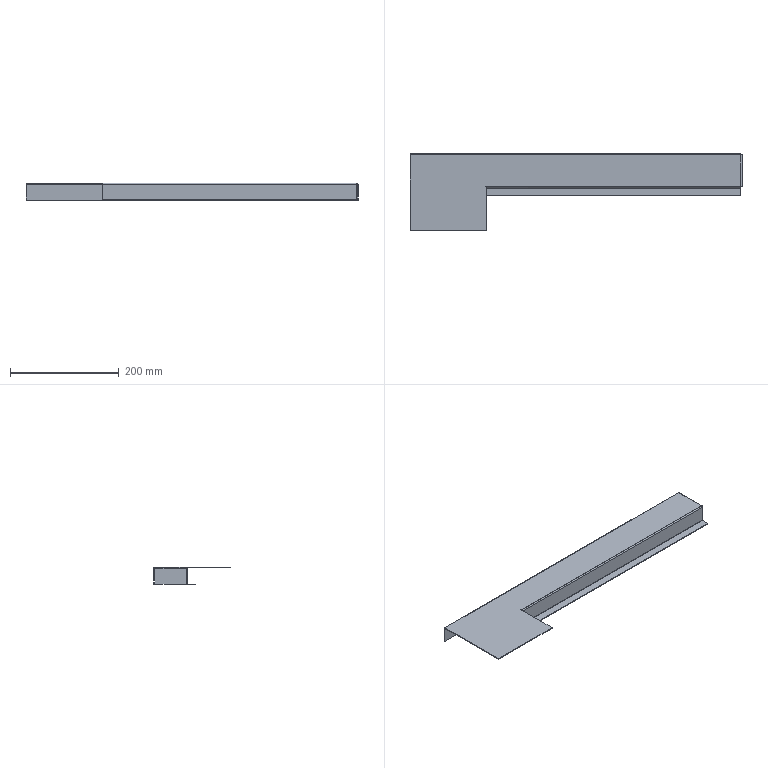Part | NX | 1 solid | 44 faces | box 611.5 x 141.5 x 33 mm | volume 135505 mm3 | plane 32 | cylinder 8 | spline 4 | commonest cylinder face diameters 1.473 x4 4.473 x4
STEP:
#1=CARTESIAN_POINT('',(304.293,-31.5,-30.763));
#2=VERTEX_POINT('',#1);
#3=CARTESIAN_POINT('',(304.293,-31.5,-2.237));
#4=VERTEX_POINT('',#3);
#5=CARTESIAN_POINT('',(304.293,-31.5,0.));
#6=DIRECTION('',(0.,0.,1.));
#7=VECTOR('',#6,1000.);
#8=LINE('',#5,#7);
#9=EDGE_CURVE('',#2,#4,#8,.T.);
#10=ORIENTED_EDGE('',*,*,#9,.F.);
#11=CARTESIAN_POINT('',(304.293,-30.,-30.763));
#12=VERTEX_POINT('',#11);
#13=CARTESIAN_POINT('',(304.293,-31.5,-30.763));
#14=DIRECTION('',(0.,1.,0.));
#15=VECTOR('',#14,1000.);
#16=LINE('',#13,#15);
#17=EDGE_CURVE('',#2,#12,#16,.T.);
#18=ORIENTED_EDGE('',*,*,#17,.T.);
#19=CARTESIAN_POINT('',(304.293,-30.,-2.237));
#20=VERTEX_POINT('',#19);
#21=CARTESIAN_POINT('',(304.293,-30.,-1.5));
#22=DIRECTION('',(0.,0.,-1.));
#23=VECTOR('',#22,1000.);
#24=LINE('',#21,#23);
#25=EDGE_CURVE('',#20,#12,#24,.T.);
#26=ORIENTED_EDGE('',*,*,#25,.F.);
#27=CARTESIAN_POINT('',(304.293,-30.,-2.237));
#28=DIRECTION('',(0.,1.,0.));
#29=VECTOR('',#28,1000.);
#30=LINE('',#27,#29);
#31=EDGE_CURVE('',#4,#20,#30,.T.);
#32=ORIENTED_EDGE('',*,*,#31,.F.);
#33=EDGE_LOOP('',(#10,#18,#26,#32));
#34=FACE_BOUND('',#33,.T.);
#35=CARTESIAN_POINT('',(304.293,-30.,-1.5));
#36=DIRECTION('',(1.,0.,0.));
#37=DIRECTION('',(0.,0.,-1.));
#38=AXIS2_PLACEMENT_3D('',#35,#36,#37);
#39=PLANE('',#38);
#40=ADVANCED_FACE('',(#34),#39,.T.);
#41=CARTESIAN_POINT('',(-165.,-31.5,-30.763));
#42=VERTEX_POINT('',#41);
#43=CARTESIAN_POINT('',(-165.,-31.5,-2.237));
#44=VERTEX_POINT('',#43);
#45=CARTESIAN_POINT('',(-165.,-31.5,-1.5));
#46=DIRECTION('',(0.,0.,1.));
#47=VECTOR('',#46,1000.);
#48=LINE('',#45,#47);
#49=EDGE_CURVE('',#42,#44,#48,.T.);
#50=ORIENTED_EDGE('',*,*,#49,.F.);
#51=CARTESIAN_POINT('',(304.293,-31.5,-30.763));
#52=DIRECTION('',(1.,0.,0.));
#53=VECTOR('',#52,1000.);
#54=LINE('',#51,#53);
#55=EDGE_CURVE('',#2,#42,#54,.F.);
#56=ORIENTED_EDGE('',*,*,#55,.F.);
#57=ORIENTED_EDGE('',*,*,#9,.T.);
#58=CARTESIAN_POINT('',(0.,-31.5,-2.237));
#59=DIRECTION('',(-1.,0.,0.));
#60=VECTOR('',#59,1000.);
#61=LINE('',#58,#60);
#62=EDGE_CURVE('',#4,#44,#61,.T.);
#63=ORIENTED_EDGE('',*,*,#62,.T.);
#64=EDGE_LOOP('',(#50,#56,#57,#63));
#65=FACE_BOUND('',#64,.T.);
#66=CARTESIAN_POINT('',(0.,-31.5,0.));
#67=DIRECTION('',(0.,-1.,0.));
#68=DIRECTION('',(0.,0.,-1.));
#69=AXIS2_PLACEMENT_3D('',#66,#67,#68);
#70=PLANE('',#69);
#71=ADVANCED_FACE('',(#65),#70,.T.);
#72=CARTESIAN_POINT('',(-165.,-30.,-30.763));
#73=VERTEX_POINT('',#72);
#74=CARTESIAN_POINT('',(304.293,-30.,-30.763));
#75=DIRECTION('',(1.,0.,0.));
#76=VECTOR('',#75,1000.);
#77=LINE('',#74,#76);
#78=EDGE_CURVE('',#12,#73,#77,.F.);
#79=ORIENTED_EDGE('',*,*,#78,.T.);
#80=CARTESIAN_POINT('',(-165.,-30.,-2.237));
#81=VERTEX_POINT('',#80);
#82=CARTESIAN_POINT('',(-165.,-30.,-1.5));
#83=DIRECTION('',(0.,0.,1.));
#84=VECTOR('',#83,1000.);
#85=LINE('',#82,#84);
#86=EDGE_CURVE('',#73,#81,#85,.T.);
#87=ORIENTED_EDGE('',*,*,#86,.T.);
#88=CARTESIAN_POINT('',(305.,-30.,-2.237));
#89=DIRECTION('',(-1.,0.,0.));
#90=VECTOR('',#89,1000.);
#91=LINE('',#88,#90);
#92=EDGE_CURVE('',#20,#81,#91,.T.);
#93=ORIENTED_EDGE('',*,*,#92,.F.);
#94=ORIENTED_EDGE('',*,*,#25,.T.);
#95=EDGE_LOOP('',(#79,#87,#93,#94));
#96=FACE_BOUND('',#95,.T.);
#97=CARTESIAN_POINT('',(0.,-30.,0.));
#98=DIRECTION('',(0.,-1.,0.));
#99=DIRECTION('',(0.,0.,-1.));
#100=AXIS2_PLACEMENT_3D('',#97,#98,#99);
#101=PLANE('',#100);
#102=ADVANCED_FACE('',(#96),#101,.F.);
#103=CARTESIAN_POINT('',(-305.,29.263,-1.5));
#104=VERTEX_POINT('',#103);
#105=CARTESIAN_POINT('',(-305.,-110.,-1.5));
#106=VERTEX_POINT('',#105);
#107=CARTESIAN_POINT('',(-305.,-30.,-1.5));
#108=DIRECTION('',(0.,-1.,0.));
#109=VECTOR('',#108,1000.);
#110=LINE('',#107,#109);
#111=EDGE_CURVE('',#104,#106,#110,.T.);
#112=ORIENTED_EDGE('',*,*,#111,.F.);
#113=CARTESIAN_POINT('',(304.263,29.263,-1.5));
#114=VERTEX_POINT('',#113);
#115=CARTESIAN_POINT('',(304.293,29.263,-1.5));
#116=DIRECTION('',(1.,0.,0.));
#117=VECTOR('',#116,1000.);
#118=LINE('',#115,#117);
#119=EDGE_CURVE('',#114,#104,#118,.F.);
#120=ORIENTED_EDGE('',*,*,#119,.F.);
#121=CARTESIAN_POINT('',(304.263,-29.263,-1.5));
#122=VERTEX_POINT('',#121);
#123=CARTESIAN_POINT('',(304.263,-29.293,-1.5));
#124=DIRECTION('',(0.,-1.,0.));
#125=VECTOR('',#124,1000.);
#126=LINE('',#123,#125);
#127=EDGE_CURVE('',#122,#114,#126,.F.);
#128=ORIENTED_EDGE('',*,*,#127,.F.);
#129=CARTESIAN_POINT('',(-165.,-29.263,-1.5));
#130=VERTEX_POINT('',#129);
#131=CARTESIAN_POINT('',(-165.,-29.263,-1.5));
#132=DIRECTION('',(-1.,0.,0.));
#133=VECTOR('',#132,1000.);
#134=LINE('',#131,#133);
#135=EDGE_CURVE('',#130,#122,#134,.F.);
#136=ORIENTED_EDGE('',*,*,#135,.F.);
#137=CARTESIAN_POINT('',(-165.,-28.513,-1.5));
#138=VERTEX_POINT('',#137);
#139=CARTESIAN_POINT('',(-165.,-28.513,-1.5));
#140=DIRECTION('',(0.,-1.,0.));
#141=VECTOR('',#140,1000.);
#142=LINE('',#139,#141);
#143=EDGE_CURVE('',#138,#130,#142,.T.);
#144=ORIENTED_EDGE('',*,*,#143,.F.);
#145=CARTESIAN_POINT('',(-165.75,-28.513,-1.5));
#146=VERTEX_POINT('',#145);
#147=CARTESIAN_POINT('',(-165.75,-28.513,-1.5));
#148=DIRECTION('',(1.,0.,0.));
#149=VECTOR('',#148,1000.);
#150=LINE('',#147,#149);
#151=EDGE_CURVE('',#146,#138,#150,.T.);
#152=ORIENTED_EDGE('',*,*,#151,.F.);
#153=CARTESIAN_POINT('',(-165.75,-30.,-1.5));
#154=VERTEX_POINT('',#153);
#155=CARTESIAN_POINT('',(-165.75,-30.,-1.5));
#156=DIRECTION('',(0.,1.,0.));
#157=VECTOR('',#156,1000.);
#158=LINE('',#155,#157);
#159=EDGE_CURVE('',#154,#146,#158,.T.);
#160=ORIENTED_EDGE('',*,*,#159,.F.);
#161=CARTESIAN_POINT('',(-165.,-30.,-1.5));
#162=VERTEX_POINT('',#161);
#163=CARTESIAN_POINT('',(-165.,-30.,-1.5));
#164=DIRECTION('',(-1.,0.,0.));
#165=VECTOR('',#164,1000.);
#166=LINE('',#163,#165);
#167=EDGE_CURVE('',#162,#154,#166,.T.);
#168=ORIENTED_EDGE('',*,*,#167,.F.);
#169=CARTESIAN_POINT('',(-165.,-110.,-1.5));
#170=VERTEX_POINT('',#169);
#171=CARTESIAN_POINT('',(-165.,-30.,-1.5));
#172=DIRECTION('',(0.,1.,0.));
#173=VECTOR('',#172,1000.);
#174=LINE('',#171,#173);
#175=EDGE_CURVE('',#170,#162,#174,.T.);
#176=ORIENTED_EDGE('',*,*,#175,.F.);
#177=CARTESIAN_POINT('',(-165.,-110.,-1.5));
#178=DIRECTION('',(1.,0.,0.));
#179=VECTOR('',#178,1000.);
#180=LINE('',#177,#179);
#181=EDGE_CURVE('',#106,#170,#180,.T.);
#182=ORIENTED_EDGE('',*,*,#181,.F.);
#183=EDGE_LOOP('',(#112,#120,#128,#136,#144,#152,#160,#168,#176,#182));
#184=FACE_BOUND('',#183,.T.);
#185=CARTESIAN_POINT('',(0.,0.,-1.5));
#186=DIRECTION('',(0.,0.,-1.));
#187=DIRECTION('',(-1.,0.,0.));
#188=AXIS2_PLACEMENT_3D('',#185,#186,#187);
#189=PLANE('',#188);
#190=ADVANCED_FACE('',(#184),#189,.T.);
#191=CARTESIAN_POINT('',(304.263,29.263,0.));
#192=VERTEX_POINT('',#191);
#193=CARTESIAN_POINT('',(-305.,29.263,0.));
#194=VERTEX_POINT('',#193);
#195=CARTESIAN_POINT('',(304.293,29.263,0.));
#196=DIRECTION('',(1.,0.,0.));
#197=VECTOR('',#196,1000.);
#198=LINE('',#195,#197);
#199=EDGE_CURVE('',#192,#194,#198,.F.);
#200=ORIENTED_EDGE('',*,*,#199,.T.);
#201=CARTESIAN_POINT('',(-305.,-110.,0.));
#202=VERTEX_POINT('',#201);
#203=CARTESIAN_POINT('',(-305.,-30.,0.));
#204=DIRECTION('',(0.,-1.,0.));
#205=VECTOR('',#204,1000.);
#206=LINE('',#203,#205);
#207=EDGE_CURVE('',#194,#202,#206,.T.);
#208=ORIENTED_EDGE('',*,*,#207,.T.);
#209=CARTESIAN_POINT('',(-165.,-110.,0.));
#210=VERTEX_POINT('',#209);
#211=CARTESIAN_POINT('',(-165.,-110.,0.));
#212=DIRECTION('',(1.,0.,0.));
#213=VECTOR('',#212,1000.);
#214=LINE('',#211,#213);
#215=EDGE_CURVE('',#202,#210,#214,.T.);
#216=ORIENTED_EDGE('',*,*,#215,.T.);
#217=CARTESIAN_POINT('',(-165.,-30.,0.));
#218=VERTEX_POINT('',#217);
#219=CARTESIAN_POINT('',(-165.,-30.,0.));
#220=DIRECTION('',(0.,1.,0.));
#221=VECTOR('',#220,1000.);
#222=LINE('',#219,#221);
#223=EDGE_CURVE('',#210,#218,#222,.T.);
#224=ORIENTED_EDGE('',*,*,#223,.T.);
#225=CARTESIAN_POINT('',(-165.75,-30.,0.));
#226=VERTEX_POINT('',#225);
#227=CARTESIAN_POINT('',(0.,-30.,0.));
#228=DIRECTION('',(1.,0.,0.));
#229=VECTOR('',#228,1000.);
#230=LINE('',#227,#229);
#231=EDGE_CURVE('',#226,#218,#230,.T.);
#232=ORIENTED_EDGE('',*,*,#231,.F.);
#233=CARTESIAN_POINT('',(-165.75,-28.513,0.));
#234=VERTEX_POINT('',#233);
#235=CARTESIAN_POINT('',(-165.75,0.,0.));
#236=DIRECTION('',(0.,-1.,0.));
#237=VECTOR('',#236,1000.);
#238=LINE('',#235,#237);
#239=EDGE_CURVE('',#234,#226,#238,.T.);
#240=ORIENTED_EDGE('',*,*,#239,.F.);
#241=CARTESIAN_POINT('',(-165.,-28.513,0.));
#242=VERTEX_POINT('',#241);
#243=CARTESIAN_POINT('',(0.,-28.513,0.));
#244=DIRECTION('',(-1.,0.,0.));
#245=VECTOR('',#244,1000.);
#246=LINE('',#243,#245);
#247=EDGE_CURVE('',#242,#234,#246,.T.);
#248=ORIENTED_EDGE('',*,*,#247,.F.);
#249=CARTESIAN_POINT('',(-165.,-29.263,0.));
#250=VERTEX_POINT('',#249);
#251=CARTESIAN_POINT('',(-165.,0.,0.));
#252=DIRECTION('',(0.,1.,0.));
#253=VECTOR('',#252,1000.);
#254=LINE('',#251,#253);
#255=EDGE_CURVE('',#250,#242,#254,.T.);
#256=ORIENTED_EDGE('',*,*,#255,.F.);
#257=CARTESIAN_POINT('',(304.263,-29.263,0.));
#258=VERTEX_POINT('',#257);
#259=CARTESIAN_POINT('',(-165.,-29.263,0.));
#260=DIRECTION('',(-1.,0.,0.));
#261=VECTOR('',#260,1000.);
#262=LINE('',#259,#261);
#263=EDGE_CURVE('',#250,#258,#262,.F.);
#264=ORIENTED_EDGE('',*,*,#263,.T.);
#265=CARTESIAN_POINT('',(304.263,-29.293,0.));
#266=DIRECTION('',(0.,-1.,0.));
#267=VECTOR('',#266,1000.);
#268=LINE('',#265,#267);
#269=EDGE_CURVE('',#258,#192,#268,.F.);
#270=ORIENTED_EDGE('',*,*,#269,.T.);
#271=EDGE_LOOP('',(#200,#208,#216,#224,#232,#240,#248,#256,#264,#270));
#272=FACE_BOUND('',#271,.T.);
#273=CARTESIAN_POINT('',(0.,0.,0.));
#274=DIRECTION('',(0.,0.,-1.));
#275=DIRECTION('',(-1.,0.,0.));
#276=AXIS2_PLACEMENT_3D('',#273,#274,#275);
#277=PLANE('',#276);
#278=ADVANCED_FACE('',(#272),#277,.F.);
#279=CARTESIAN_POINT('',(-305.,29.263,-1.5));
#280=DIRECTION('',(0.,0.,1.));
#281=VECTOR('',#280,1000.);
#282=LINE('',#279,#281);
#283=EDGE_CURVE('',#104,#194,#282,.T.);
#284=ORIENTED_EDGE('',*,*,#283,.F.);
#285=ORIENTED_EDGE('',*,*,#111,.T.);
#286=CARTESIAN_POINT('',(-305.,-110.,-1.5));
#287=DIRECTION('',(0.,0.,1.));
#288=VECTOR('',#287,1000.);
#289=LINE('',#286,#288);
#290=EDGE_CURVE('',#106,#202,#289,.T.);
#291=ORIENTED_EDGE('',*,*,#290,.T.);
#292=ORIENTED_EDGE('',*,*,#207,.F.);
#293=EDGE_LOOP('',(#284,#285,#291,#292));
#294=FACE_BOUND('',#293,.T.);
#295=CARTESIAN_POINT('',(-305.,-30.,-1.5));
#296=DIRECTION('',(-1.,0.,0.));
#297=DIRECTION('',(0.,0.,1.));
#298=AXIS2_PLACEMENT_3D('',#295,#296,#297);
#299=PLANE('',#298);
#300=ADVANCED_FACE('',(#294),#299,.T.);
#301=ORIENTED_EDGE('',*,*,#223,.F.);
#302=CARTESIAN_POINT('',(-165.,-110.,-1.5));
#303=DIRECTION('',(0.,0.,1.));
#304=VECTOR('',#303,1000.);
#305=LINE('',#302,#304);
#306=EDGE_CURVE('',#170,#210,#305,.T.);
#307=ORIENTED_EDGE('',*,*,#306,.F.);
#308=ORIENTED_EDGE('',*,*,#175,.T.);
#309=CARTESIAN_POINT('',(-165.,-30.,-1.5));
#310=DIRECTION('',(0.,0.,1.));
#311=VECTOR('',#310,1000.);
#312=LINE('',#309,#311);
#313=EDGE_CURVE('',#162,#218,#312,.T.);
#314=ORIENTED_EDGE('',*,*,#313,.T.);
#315=EDGE_LOOP('',(#301,#307,#308,#314));
#316=FACE_BOUND('',#315,.T.);
#317=CARTESIAN_POINT('',(-165.,-30.,-1.5));
#318=DIRECTION('',(1.,0.,0.));
#319=DIRECTION('',(0.,0.,-1.));
#320=AXIS2_PLACEMENT_3D('',#317,#318,#319);
#321=PLANE('',#320);
#322=ADVANCED_FACE('',(#316),#321,.T.);
#323=ORIENTED_EDGE('',*,*,#215,.F.);
#324=ORIENTED_EDGE('',*,*,#290,.F.);
#325=ORIENTED_EDGE('',*,*,#181,.T.);
#326=ORIENTED_EDGE('',*,*,#306,.T.);
#327=EDGE_LOOP('',(#323,#324,#325,#326));
#328=FACE_BOUND('',#327,.T.);
#329=CARTESIAN_POINT('',(-165.,-110.,-1.5));
#330=DIRECTION('',(0.,-1.,0.));
#331=DIRECTION('',(1.,0.,0.));
#332=AXIS2_PLACEMENT_3D('',#329,#330,#331);
#333=PLANE('',#332);
#334=ADVANCED_FACE('',(#328),#333,.T.);
#335=CARTESIAN_POINT('',(-165.75,-28.513,-1.5));
#336=DIRECTION('',(0.,0.,1.));
#337=VECTOR('',#336,1000.);
#338=LINE('',#335,#337);
#339=EDGE_CURVE('',#146,#234,#338,.T.);
#340=ORIENTED_EDGE('',*,*,#339,.T.);
#341=ORIENTED_EDGE('',*,*,#239,.T.);
#342=CARTESIAN_POINT('',(-165.75,-30.,-1.5));
#343=DIRECTION('',(0.,0.,1.));
#344=VECTOR('',#343,1000.);
#345=LINE('',#342,#344);
#346=EDGE_CURVE('',#154,#226,#345,.T.);
#347=ORIENTED_EDGE('',*,*,#346,.F.);
#348=ORIENTED_EDGE('',*,*,#159,.T.);
#349=EDGE_LOOP('',(#340,#341,#347,#348));
#350=FACE_BOUND('',#349,.T.);
#351=CARTESIAN_POINT('',(-165.75,-30.,-1.5));
#352=DIRECTION('',(1.,0.,0.));
#353=DIRECTION('',(0.,0.,-1.));
#354=AXIS2_PLACEMENT_3D('',#351,#352,#353);
#355=PLANE('',#354);
#356=ADVANCED_FACE('',(#350),#355,.T.);
#357=CARTESIAN_POINT('',(-165.,-28.513,-1.5));
#358=DIRECTION('',(0.,0.,1.));
#359=VECTOR('',#358,1000.);
#360=LINE('',#357,#359);
#361=EDGE_CURVE('',#138,#242,#360,.T.);
#362=ORIENTED_EDGE('',*,*,#361,.T.);
#363=ORIENTED_EDGE('',*,*,#247,.T.);
#364=ORIENTED_EDGE('',*,*,#339,.F.);
#365=ORIENTED_EDGE('',*,*,#151,.T.);
#366=EDGE_LOOP('',(#362,#363,#364,#365));
#367=FACE_BOUND('',#366,.T.);
#368=CARTESIAN_POINT('',(-165.75,-28.513,-1.5));
#369=DIRECTION('',(0.,-1.,0.));
#370=DIRECTION('',(0.,0.,-1.));
#371=AXIS2_PLACEMENT_3D('',#368,#369,#370);
#372=PLANE('',#371);
#373=ADVANCED_FACE('',(#367),#372,.T.);
#374=CARTESIAN_POINT('',(-165.,-29.263,-1.5));
#375=DIRECTION('',(0.,0.,1.));
#376=VECTOR('',#375,1000.);
#377=LINE('',#374,#376);
#378=EDGE_CURVE('',#130,#250,#377,.T.);
#379=ORIENTED_EDGE('',*,*,#378,.T.);
#380=ORIENTED_EDGE('',*,*,#255,.T.);
#381=ORIENTED_EDGE('',*,*,#361,.F.);
#382=ORIENTED_EDGE('',*,*,#143,.T.);
#383=EDGE_LOOP('',(#379,#380,#381,#382));
#384=FACE_BOUND('',#383,.T.);
#385=CARTESIAN_POINT('',(-165.,-28.513,-1.5));
#386=DIRECTION('',(-1.,0.,0.));
#387=DIRECTION('',(0.,0.,1.));
#388=AXIS2_PLACEMENT_3D('',#385,#386,#387);
#389=PLANE('',#388);
#390=ADVANCED_FACE('',(#384),#389,.T.);
#391=ORIENTED_EDGE('',*,*,#346,.T.);
#392=ORIENTED_EDGE('',*,*,#231,.T.);
#393=ORIENTED_EDGE('',*,*,#313,.F.);
#394=ORIENTED_EDGE('',*,*,#167,.T.);
#395=EDGE_LOOP('',(#391,#392,#393,#394));
#396=FACE_BOUND('',#395,.T.);
#397=CARTESIAN_POINT('',(-165.,-30.,-1.5));
#398=DIRECTION('',(0.,1.,0.));
#399=DIRECTION('',(0.,0.,1.));
#400=AXIS2_PLACEMENT_3D('',#397,#398,#399);
#401=PLANE('',#400);
#402=ADVANCED_FACE('',(#396),#401,.T.);
#403=ORIENTED_EDGE('',*,*,#31,.T.);
#404=CARTESIAN_POINT('',(304.263,-29.263,-1.5));
#405=CARTESIAN_POINT('',(304.273,-29.649,-1.5));
#406=CARTESIAN_POINT('',(304.283,-30.,-1.851));
#407=CARTESIAN_POINT('',(304.293,-30.,-2.237));
#408=B_SPLINE_CURVE_WITH_KNOTS('',3,(#404,#405,#406,#407),.UNSPECIFIED.,.F.,.F.,(4,4),(0.,1.),.UNSPECIFIED.);
#409=EDGE_CURVE('',#122,#20,#408,.T.);
#410=ORIENTED_EDGE('',*,*,#409,.F.);
#411=CARTESIAN_POINT('',(304.263,-29.263,-1.5));
#412=DIRECTION('',(0.,0.,1.));
#413=VECTOR('',#412,1000.);
#414=LINE('',#411,#413);
#415=EDGE_CURVE('',#122,#258,#414,.T.);
#416=ORIENTED_EDGE('',*,*,#415,.T.);
#417=CARTESIAN_POINT('',(304.263,-29.263,0.));
#418=CARTESIAN_POINT('',(304.268,-29.849,0.));
#419=CARTESIAN_POINT('',(304.278,-31.015,-0.4846));
#420=CARTESIAN_POINT('',(304.288,-31.5,-1.651));
#421=CARTESIAN_POINT('',(304.293,-31.5,-2.237));
#422=B_SPLINE_CURVE_WITH_KNOTS('',3,(#417,#418,#419,#420,#421),.UNSPECIFIED.,.F.,.F.,(4,1,4),(0.,0.5,1.),.UNSPECIFIED.);
#423=EDGE_CURVE('',#258,#4,#422,.T.);
#424=ORIENTED_EDGE('',*,*,#423,.T.);
#425=EDGE_LOOP('',(#403,#410,#416,#424));
#426=FACE_BOUND('',#425,.T.);
#427=CARTESIAN_POINT('',(304.263,-29.263,0.015));
#428=CARTESIAN_POINT('',(304.266,-29.558,0.015));
#429=CARTESIAN_POINT('',(304.268,-29.853,-0.0436));
#430=CARTESIAN_POINT('',(304.273,-30.397,-0.2692));
#431=CARTESIAN_POINT('',(304.276,-30.647,-0.4361));
#432=CARTESIAN_POINT('',(304.281,-31.064,-0.8529));
#433=CARTESIAN_POINT('',(304.283,-31.231,-1.103));
#434=CARTESIAN_POINT('',(304.288,-31.456,-1.647));
#435=CARTESIAN_POINT('',(304.29,-31.515,-1.942));
#436=CARTESIAN_POINT('',(304.293,-31.515,-2.237));
#437=CARTESIAN_POINT('',(304.263,-29.263,0.));
#438=CARTESIAN_POINT('',(304.266,-29.556,0.));
#439=CARTESIAN_POINT('',(304.268,-29.849,-0.05821));
#440=CARTESIAN_POINT('',(304.273,-30.39,-0.2823));
#441=CARTESIAN_POINT('',(304.276,-30.638,-0.4481));
#442=CARTESIAN_POINT('',(304.281,-31.052,-0.8621));
#443=CARTESIAN_POINT('',(304.283,-31.218,-1.11));
#444=CARTESIAN_POINT('',(304.288,-31.442,-1.651));
#445=CARTESIAN_POINT('',(304.29,-31.5,-1.944));
#446=CARTESIAN_POINT('',(304.293,-31.5,-2.237));
#447=CARTESIAN_POINT('',(304.263,-29.263,-1.5));
#448=CARTESIAN_POINT('',(304.266,-29.36,-1.5));
#449=CARTESIAN_POINT('',(304.268,-29.456,-1.519));
#450=CARTESIAN_POINT('',(304.273,-29.634,-1.593));
#451=CARTESIAN_POINT('',(304.276,-29.716,-1.648));
#452=CARTESIAN_POINT('',(304.281,-29.852,-1.784));
#453=CARTESIAN_POINT('',(304.283,-29.907,-1.866));
#454=CARTESIAN_POINT('',(304.288,-29.981,-2.044));
#455=CARTESIAN_POINT('',(304.29,-30.,-2.14));
#456=CARTESIAN_POINT('',(304.293,-30.,-2.237));
#457=CARTESIAN_POINT('',(304.263,-29.263,-1.515));
#458=CARTESIAN_POINT('',(304.266,-29.358,-1.515));
#459=CARTESIAN_POINT('',(304.268,-29.452,-1.534));
#460=CARTESIAN_POINT('',(304.273,-29.627,-1.606));
#461=CARTESIAN_POINT('',(304.276,-29.707,-1.66));
#462=CARTESIAN_POINT('',(304.281,-29.84,-1.793));
#463=CARTESIAN_POINT('',(304.283,-29.894,-1.873));
#464=CARTESIAN_POINT('',(304.288,-29.966,-2.048));
#465=CARTESIAN_POINT('',(304.29,-29.985,-2.142));
#466=CARTESIAN_POINT('',(304.293,-29.985,-2.237));
#467=B_SPLINE_SURFACE_WITH_KNOTS('',1,3,((#427,#428,#429,#430,#431,#432,#433,#434,#435,#436),(#437,#438,#439,#440,#441,#442,#443,#444,#445,#446),(#447,#448,#449,#450,#451,#452,#453,#454,#455,#456),(#457,#458,#459,#460,#461,#462,#463,#464,#465,#466)),.RULED_SURF.,.F.,.F.,.F.,(2,1,1,2),(4,2,2,2,4),(-0.01,0.,1.,1.01),(0.,0.25,0.5,0.75,1.),.UNSPECIFIED.);
#468=ADVANCED_FACE('',(#426),#467,.F.);
#469=CARTESIAN_POINT('',(-165.,-29.263,-2.237));
#470=DIRECTION('',(-1.,0.,0.));
#471=DIRECTION('',(0.,0.,1.));
#472=AXIS2_PLACEMENT_3D('',#469,#470,#471);
#473=CIRCLE('',#472,0.7366);
#474=EDGE_CURVE('',#81,#130,#473,.T.);
#475=ORIENTED_EDGE('',*,*,#474,.F.);
#476=CARTESIAN_POINT('',(-165.,-30.,-2.237));
#477=DIRECTION('',(0.,-1.,0.));
#478=VECTOR('',#477,1000.);
#479=LINE('',#476,#478);
#480=EDGE_CURVE('',#81,#44,#479,.T.);
#481=ORIENTED_EDGE('',*,*,#480,.T.);
#482=CARTESIAN_POINT('',(-165.,-29.263,-2.237));
#483=DIRECTION('',(-1.,0.,0.));
#484=DIRECTION('',(0.,0.,1.));
#485=AXIS2_PLACEMENT_3D('',#482,#483,#484);
#486=CIRCLE('',#485,2.237);
#487=EDGE_CURVE('',#44,#250,#486,.T.);
#488=ORIENTED_EDGE('',*,*,#487,.T.);
#489=ORIENTED_EDGE('',*,*,#378,.F.);
#490=EDGE_LOOP('',(#475,#481,#488,#489));
#491=FACE_BOUND('',#490,.T.);
#492=CARTESIAN_POINT('',(-165.,-29.263,-2.237));
#493=DIRECTION('',(1.,0.,0.));
#494=DIRECTION('',(0.,0.,-1.));
#495=AXIS2_PLACEMENT_3D('',#492,#493,#494);
#496=PLANE('',#495);
#497=ADVANCED_FACE('',(#491),#496,.F.);
#498=ORIENTED_EDGE('',*,*,#263,.F.);
#499=ORIENTED_EDGE('',*,*,#487,.F.);
#500=ORIENTED_EDGE('',*,*,#62,.F.);
#501=ORIENTED_EDGE('',*,*,#423,.F.);
#502=EDGE_LOOP('',(#498,#499,#500,#501));
#503=FACE_BOUND('',#502,.T.);
#504=CARTESIAN_POINT('',(-165.,-29.263,-2.237));
#505=DIRECTION('',(-1.,0.,0.));
#506=DIRECTION('',(0.,-1.,0.));
#507=AXIS2_PLACEMENT_3D('',#504,#505,#506);
#508=CYLINDRICAL_SURFACE('',#507,2.237);
#509=ADVANCED_FACE('',(#503),#508,.T.);
#510=ORIENTED_EDGE('',*,*,#135,.T.);
#511=ORIENTED_EDGE('',*,*,#409,.T.);
#512=ORIENTED_EDGE('',*,*,#92,.T.);
#513=ORIENTED_EDGE('',*,*,#474,.T.);
#514=EDGE_LOOP('',(#510,#511,#512,#513));
#515=FACE_BOUND('',#514,.T.);
#516=CARTESIAN_POINT('',(-165.,-29.263,-2.237));
#517=DIRECTION('',(-1.,0.,0.));
#518=DIRECTION('',(0.,-1.,0.));
#519=AXIS2_PLACEMENT_3D('',#516,#517,#518);
#520=CYLINDRICAL_SURFACE('',#519,0.7366);
#521=ADVANCED_FACE('',(#515),#520,.F.);
#522=CARTESIAN_POINT('',(-165.,-31.5,-30.763));
#523=DIRECTION('',(0.,1.,0.));
#524=VECTOR('',#523,1000.);
#525=LINE('',#522,#524);
#526=EDGE_CURVE('',#42,#73,#525,.T.);
#527=ORIENTED_EDGE('',*,*,#526,.F.);
#528=ORIENTED_EDGE('',*,*,#49,.T.);
#529=ORIENTED_EDGE('',*,*,#480,.F.);
#530=ORIENTED_EDGE('',*,*,#86,.F.);
#531=EDGE_LOOP('',(#527,#528,#529,#530));
#532=FACE_BOUND('',#531,.T.);
#533=CARTESIAN_POINT('',(-165.,-31.5,-1.5));
#534=DIRECTION('',(-1.,0.,0.));
#535=DIRECTION('',(0.,0.,1.));
#536=AXIS2_PLACEMENT_3D('',#533,#534,#535);
#537=PLANE('',#536);
#538=ADVANCED_FACE('',(#532),#537,.T.);
#539=CARTESIAN_POINT('',(306.5,29.293,-2.237));
#540=VERTEX_POINT('',#539);
#541=CARTESIAN_POINT('',(305.,29.293,-2.237));
#542=VERTEX_POINT('',#541);
#543=CARTESIAN_POINT('',(305.,29.293,-2.237));
#544=DIRECTION('',(-1.,0.,0.));
#545=VECTOR('',#544,1000.);
#546=LINE('',#543,#545);
#547=EDGE_CURVE('',#540,#542,#546,.T.);
#548=ORIENTED_EDGE('',*,*,#547,.T.);
#549=CARTESIAN_POINT('',(304.263,29.263,-1.5));
#550=CARTESIAN_POINT('',(304.649,29.273,-1.5));
#551=CARTESIAN_POINT('',(305.,29.283,-1.851));
#552=CARTESIAN_POINT('',(305.,29.293,-2.237));
#553=B_SPLINE_CURVE_WITH_KNOTS('',3,(#549,#550,#551,#552),.UNSPECIFIED.,.F.,.F.,(4,4),(0.,1.),.UNSPECIFIED.);
#554=EDGE_CURVE('',#114,#542,#553,.T.);
#555=ORIENTED_EDGE('',*,*,#554,.F.);
#556=CARTESIAN_POINT('',(304.263,29.263,-1.5));
#557=DIRECTION('',(0.,0.,1.));
#558=VECTOR('',#557,1000.);
#559=LINE('',#556,#558);
#560=EDGE_CURVE('',#114,#192,#559,.T.);
#561=ORIENTED_EDGE('',*,*,#560,.T.);
#562=CARTESIAN_POINT('',(304.263,29.263,0.));
#563=CARTESIAN_POINT('',(304.849,29.268,0.));
#564=CARTESIAN_POINT('',(306.015,29.278,-0.4846));
#565=CARTESIAN_POINT('',(306.5,29.288,-1.651));
#566=CARTESIAN_POINT('',(306.5,29.293,-2.237));
#567=B_SPLINE_CURVE_WITH_KNOTS('',3,(#562,#563,#564,#565,#566),.UNSPECIFIED.,.F.,.F.,(4,1,4),(0.,0.5,1.),.UNSPECIFIED.);
#568=EDGE_CURVE('',#192,#540,#567,.T.);
#569=ORIENTED_EDGE('',*,*,#568,.T.);
#570=EDGE_LOOP('',(#548,#555,#561,#569));
#571=FACE_BOUND('',#570,.T.);
#572=CARTESIAN_POINT('',(304.263,29.263,0.015));
#573=CARTESIAN_POINT('',(304.558,29.266,0.015));
#574=CARTESIAN_POINT('',(304.853,29.268,-0.0436));
#575=CARTESIAN_POINT('',(305.397,29.273,-0.2692));
#576=CARTESIAN_POINT('',(305.647,29.276,-0.4361));
#577=CARTESIAN_POINT('',(306.064,29.281,-0.8529));
#578=CARTESIAN_POINT('',(306.231,29.283,-1.103));
#579=CARTESIAN_POINT('',(306.456,29.288,-1.647));
#580=CARTESIAN_POINT('',(306.515,29.29,-1.942));
#581=CARTESIAN_POINT('',(306.515,29.293,-2.237));
#582=CARTESIAN_POINT('',(304.263,29.263,0.));
#583=CARTESIAN_POINT('',(304.556,29.266,0.));
#584=CARTESIAN_POINT('',(304.849,29.268,-0.05821));
#585=CARTESIAN_POINT('',(305.39,29.273,-0.2823));
#586=CARTESIAN_POINT('',(305.638,29.276,-0.4481));
#587=CARTESIAN_POINT('',(306.052,29.281,-0.8621));
#588=CARTESIAN_POINT('',(306.218,29.283,-1.11));
#589=CARTESIAN_POINT('',(306.442,29.288,-1.651));
#590=CARTESIAN_POINT('',(306.5,29.29,-1.944));
#591=CARTESIAN_POINT('',(306.5,29.293,-2.237));
#592=CARTESIAN_POINT('',(304.263,29.263,-1.5));
#593=CARTESIAN_POINT('',(304.36,29.266,-1.5));
#594=CARTESIAN_POINT('',(304.456,29.268,-1.519));
#595=CARTESIAN_POINT('',(304.634,29.273,-1.593));
#596=CARTESIAN_POINT('',(304.716,29.276,-1.648));
#597=CARTESIAN_POINT('',(304.852,29.281,-1.784));
#598=CARTESIAN_POINT('',(304.907,29.283,-1.866));
#599=CARTESIAN_POINT('',(304.981,29.288,-2.044));
#600=CARTESIAN_POINT('',(305.,29.29,-2.14));
#601=CARTESIAN_POINT('',(305.,29.293,-2.237));
#602=CARTESIAN_POINT('',(304.263,29.263,-1.515));
#603=CARTESIAN_POINT('',(304.358,29.266,-1.515));
#604=CARTESIAN_POINT('',(304.452,29.268,-1.534));
#605=CARTESIAN_POINT('',(304.627,29.273,-1.606));
#606=CARTESIAN_POINT('',(304.707,29.276,-1.66));
#607=CARTESIAN_POINT('',(304.84,29.281,-1.793));
#608=CARTESIAN_POINT('',(304.894,29.283,-1.873));
#609=CARTESIAN_POINT('',(304.966,29.288,-2.048));
#610=CARTESIAN_POINT('',(304.985,29.29,-2.142));
#611=CARTESIAN_POINT('',(304.985,29.293,-2.237));
#612=B_SPLINE_SURFACE_WITH_KNOTS('',1,3,((#572,#573,#574,#575,#576,#577,#578,#579,#580,#581),(#582,#583,#584,#585,#586,#587,#588,#589,#590,#591),(#592,#593,#594,#595,#596,#597,#598,#599,#600,#601),(#602,#603,#604,#605,#606,#607,#608,#609,#610,#611)),.RULED_SURF.,.F.,.F.,.F.,(2,1,1,2),(4,2,2,2,4),(-0.01,0.,1.,1.01),(0.,0.25,0.5,0.75,1.),.UNSPECIFIED.);
#613=ADVANCED_FACE('',(#571),#612,.F.);
#614=CARTESIAN_POINT('',(305.,-29.293,-2.237));
#615=VERTEX_POINT('',#614);
#616=CARTESIAN_POINT('',(305.,-29.293,-2.237));
#617=CARTESIAN_POINT('',(305.,-29.283,-1.851));
#618=CARTESIAN_POINT('',(304.649,-29.273,-1.5));
#619=CARTESIAN_POINT('',(304.263,-29.263,-1.5));
#620=B_SPLINE_CURVE_WITH_KNOTS('',3,(#616,#617,#618,#619),.UNSPECIFIED.,.F.,.F.,(4,4),(0.,1.),.UNSPECIFIED.);
#621=EDGE_CURVE('',#615,#122,#620,.T.);
#622=ORIENTED_EDGE('',*,*,#621,.F.);
#623=CARTESIAN_POINT('',(306.5,-29.293,-2.237));
#624=VERTEX_POINT('',#623);
#625=CARTESIAN_POINT('',(305.,-29.293,-2.237));
#626=DIRECTION('',(-1.,0.,0.));
#627=VECTOR('',#626,1000.);
#628=LINE('',#625,#627);
#629=EDGE_CURVE('',#624,#615,#628,.T.);
#630=ORIENTED_EDGE('',*,*,#629,.F.);
#631=CARTESIAN_POINT('',(306.5,-29.293,-2.237));
#632=CARTESIAN_POINT('',(306.5,-29.288,-1.651));
#633=CARTESIAN_POINT('',(306.015,-29.278,-0.4846));
#634=CARTESIAN_POINT('',(304.849,-29.268,0.));
#635=CARTESIAN_POINT('',(304.263,-29.263,0.));
#636=B_SPLINE_CURVE_WITH_KNOTS('',3,(#631,#632,#633,#634,#635),.UNSPECIFIED.,.F.,.F.,(4,1,4),(0.,0.5,1.),.UNSPECIFIED.);
#637=EDGE_CURVE('',#624,#258,#636,.T.);
#638=ORIENTED_EDGE('',*,*,#637,.T.);
#639=ORIENTED_EDGE('',*,*,#415,.F.);
#640=EDGE_LOOP('',(#622,#630,#638,#639));
#641=FACE_BOUND('',#640,.T.);
#642=CARTESIAN_POINT('',(306.515,-29.293,-2.237));
#643=CARTESIAN_POINT('',(306.515,-29.29,-1.942));
#644=CARTESIAN_POINT('',(306.456,-29.288,-1.647));
#645=CARTESIAN_POINT('',(306.231,-29.283,-1.103));
#646=CARTESIAN_POINT('',(306.064,-29.281,-0.8529));
#647=CARTESIAN_POINT('',(305.647,-29.276,-0.4361));
#648=CARTESIAN_POINT('',(305.397,-29.273,-0.2692));
#649=CARTESIAN_POINT('',(304.853,-29.268,-0.0436));
#650=CARTESIAN_POINT('',(304.558,-29.266,0.015));
#651=CARTESIAN_POINT('',(304.263,-29.263,0.015));
#652=CARTESIAN_POINT('',(306.5,-29.293,-2.237));
#653=CARTESIAN_POINT('',(306.5,-29.29,-1.944));
#654=CARTESIAN_POINT('',(306.442,-29.288,-1.651));
#655=CARTESIAN_POINT('',(306.218,-29.283,-1.11));
#656=CARTESIAN_POINT('',(306.052,-29.281,-0.8621));
#657=CARTESIAN_POINT('',(305.638,-29.276,-0.4481));
#658=CARTESIAN_POINT('',(305.39,-29.273,-0.2823));
#659=CARTESIAN_POINT('',(304.849,-29.268,-0.05821));
#660=CARTESIAN_POINT('',(304.556,-29.266,0.));
#661=CARTESIAN_POINT('',(304.263,-29.263,0.));
#662=CARTESIAN_POINT('',(305.,-29.293,-2.237));
#663=CARTESIAN_POINT('',(305.,-29.29,-2.14));
#664=CARTESIAN_POINT('',(304.981,-29.288,-2.044));
#665=CARTESIAN_POINT('',(304.907,-29.283,-1.866));
#666=CARTESIAN_POINT('',(304.852,-29.281,-1.784));
#667=CARTESIAN_POINT('',(304.716,-29.276,-1.648));
#668=CARTESIAN_POINT('',(304.634,-29.273,-1.593));
#669=CARTESIAN_POINT('',(304.456,-29.268,-1.519));
#670=CARTESIAN_POINT('',(304.36,-29.266,-1.5));
#671=CARTESIAN_POINT('',(304.263,-29.263,-1.5));
#672=CARTESIAN_POINT('',(304.985,-29.293,-2.237));
#673=CARTESIAN_POINT('',(304.985,-29.29,-2.142));
#674=CARTESIAN_POINT('',(304.966,-29.288,-2.048));
#675=CARTESIAN_POINT('',(304.894,-29.283,-1.873));
#676=CARTESIAN_POINT('',(304.84,-29.281,-1.793));
#677=CARTESIAN_POINT('',(304.707,-29.276,-1.66));
#678=CARTESIAN_POINT('',(304.627,-29.273,-1.606));
#679=CARTESIAN_POINT('',(304.452,-29.268,-1.534));
#680=CARTESIAN_POINT('',(304.358,-29.266,-1.515));
#681=CARTESIAN_POINT('',(304.263,-29.263,-1.515));
#682=B_SPLINE_SURFACE_WITH_KNOTS('',1,3,((#642,#643,#644,#645,#646,#647,#648,#649,#650,#651),(#652,#653,#654,#655,#656,#657,#658,#659,#660,#661),(#662,#663,#664,#665,#666,#667,#668,#669,#670,#671),(#672,#673,#674,#675,#676,#677,#678,#679,#680,#681)),.RULED_SURF.,.F.,.F.,.F.,(2,1,1,2),(4,2,2,2,4),(-0.01,0.,1.,1.01),(0.,0.25,0.5,0.75,1.),.UNSPECIFIED.);
#683=ADVANCED_FACE('',(#641),#682,.F.);
#684=ORIENTED_EDGE('',*,*,#269,.F.);
#685=ORIENTED_EDGE('',*,*,#637,.F.);
#686=CARTESIAN_POINT('',(306.5,0.,-2.237));
#687=DIRECTION('',(0.,1.,0.));
#688=VECTOR('',#687,1000.);
#689=LINE('',#686,#688);
#690=EDGE_CURVE('',#624,#540,#689,.T.);
#691=ORIENTED_EDGE('',*,*,#690,.T.);
#692=ORIENTED_EDGE('',*,*,#568,.F.);
#693=EDGE_LOOP('',(#684,#685,#691,#692));
#694=FACE_BOUND('',#693,.T.);
#695=CARTESIAN_POINT('',(304.263,-29.293,-2.237));
#696=DIRECTION('',(0.,-1.,0.));
#697=DIRECTION('',(1.,0.,0.));
#698=AXIS2_PLACEMENT_3D('',#695,#696,#697);
#699=CYLINDRICAL_SURFACE('',#698,2.237);
#700=ADVANCED_FACE('',(#694),#699,.T.);
#701=ORIENTED_EDGE('',*,*,#127,.T.);
#702=ORIENTED_EDGE('',*,*,#554,.T.);
#703=CARTESIAN_POINT('',(305.,30.,-2.237));
#704=DIRECTION('',(0.,-1.,0.));
#705=VECTOR('',#704,1000.);
#706=LINE('',#703,#705);
#707=EDGE_CURVE('',#542,#615,#706,.T.);
#708=ORIENTED_EDGE('',*,*,#707,.T.);
#709=ORIENTED_EDGE('',*,*,#621,.T.);
#710=EDGE_LOOP('',(#701,#702,#708,#709));
#711=FACE_BOUND('',#710,.T.);
#712=CARTESIAN_POINT('',(304.263,-29.293,-2.237));
#713=DIRECTION('',(0.,-1.,0.));
#714=DIRECTION('',(1.,0.,0.));
#715=AXIS2_PLACEMENT_3D('',#712,#713,#714);
#716=CYLINDRICAL_SURFACE('',#715,0.7366);
#717=ADVANCED_FACE('',(#711),#716,.F.);
#718=CARTESIAN_POINT('',(305.,29.293,-31.5));
#719=VERTEX_POINT('',#718);
#720=CARTESIAN_POINT('',(306.5,29.293,-31.5));
#721=VERTEX_POINT('',#720);
#722=CARTESIAN_POINT('',(306.5,29.293,-31.5));
#723=DIRECTION('',(1.,0.,0.));
#724=VECTOR('',#723,1000.);
#725=LINE('',#722,#724);
#726=EDGE_CURVE('',#719,#721,#725,.T.);
#727=ORIENTED_EDGE('',*,*,#726,.F.);
#728=CARTESIAN_POINT('',(305.,29.293,-1.5));
#729=DIRECTION('',(0.,0.,-1.));
#730=VECTOR('',#729,1000.);
#731=LINE('',#728,#730);
#732=EDGE_CURVE('',#542,#719,#731,.T.);
#733=ORIENTED_EDGE('',*,*,#732,.F.);
#734=ORIENTED_EDGE('',*,*,#547,.F.);
#735=CARTESIAN_POINT('',(306.5,29.293,0.));
#736=DIRECTION('',(0.,0.,-1.));
#737=VECTOR('',#736,1000.);
#738=LINE('',#735,#737);
#739=EDGE_CURVE('',#540,#721,#738,.T.);
#740=ORIENTED_EDGE('',*,*,#739,.T.);
#741=EDGE_LOOP('',(#727,#733,#734,#740));
#742=FACE_BOUND('',#741,.T.);
#743=CARTESIAN_POINT('',(305.,29.293,-1.5));
#744=DIRECTION('',(0.,1.,0.));
#745=DIRECTION('',(0.,0.,1.));
#746=AXIS2_PLACEMENT_3D('',#743,#744,#745);
#747=PLANE('',#746);
#748=ADVANCED_FACE('',(#742),#747,.T.);
#749=ORIENTED_EDGE('',*,*,#690,.F.);
#750=CARTESIAN_POINT('',(306.5,-29.293,-31.5));
#751=VERTEX_POINT('',#750);
#752=CARTESIAN_POINT('',(306.5,-29.293,0.));
#753=DIRECTION('',(0.,0.,-1.));
#754=VECTOR('',#753,1000.);
#755=LINE('',#752,#754);
#756=EDGE_CURVE('',#624,#751,#755,.T.);
#757=ORIENTED_EDGE('',*,*,#756,.T.);
#758=CARTESIAN_POINT('',(306.5,30.,-31.5));
#759=DIRECTION('',(0.,-1.,0.));
#760=VECTOR('',#759,1000.);
#761=LINE('',#758,#760);
#762=EDGE_CURVE('',#721,#751,#761,.T.);
#763=ORIENTED_EDGE('',*,*,#762,.F.);
#764=ORIENTED_EDGE('',*,*,#739,.F.);
#765=EDGE_LOOP('',(#749,#757,#763,#764));
#766=FACE_BOUND('',#765,.T.);
#767=CARTESIAN_POINT('',(306.5,0.,0.));
#768=DIRECTION('',(-1.,0.,0.));
#769=DIRECTION('',(0.,0.,1.));
#770=AXIS2_PLACEMENT_3D('',#767,#768,#769);
#771=PLANE('',#770);
#772=ADVANCED_FACE('',(#766),#771,.F.);
#773=CARTESIAN_POINT('',(305.,-29.293,-31.5));
#774=VERTEX_POINT('',#773);
#775=CARTESIAN_POINT('',(305.,-29.293,-1.5));
#776=DIRECTION('',(0.,0.,-1.));
#777=VECTOR('',#776,1000.);
#778=LINE('',#775,#777);
#779=EDGE_CURVE('',#615,#774,#778,.T.);
#780=ORIENTED_EDGE('',*,*,#779,.F.);
#781=ORIENTED_EDGE('',*,*,#707,.F.);
#782=ORIENTED_EDGE('',*,*,#732,.T.);
#783=CARTESIAN_POINT('',(305.,30.,-31.5));
#784=DIRECTION('',(0.,-1.,0.));
#785=VECTOR('',#784,1000.);
#786=LINE('',#783,#785);
#787=EDGE_CURVE('',#719,#774,#786,.T.);
#788=ORIENTED_EDGE('',*,*,#787,.T.);
#789=EDGE_LOOP('',(#780,#781,#782,#788));
#790=FACE_BOUND('',#789,.T.);
#791=CARTESIAN_POINT('',(305.,0.,0.));
#792=DIRECTION('',(-1.,0.,0.));
#793=DIRECTION('',(0.,0.,1.));
#794=AXIS2_PLACEMENT_3D('',#791,#792,#793);
#795=PLANE('',#794);
#796=ADVANCED_FACE('',(#790),#795,.T.);
#797=CARTESIAN_POINT('',(306.5,-29.293,-31.5));
#798=DIRECTION('',(1.,0.,0.));
#799=VECTOR('',#798,1000.);
#800=LINE('',#797,#799);
#801=EDGE_CURVE('',#774,#751,#800,.T.);
#802=ORIENTED_EDGE('',*,*,#801,.F.);
#803=ORIENTED_EDGE('',*,*,#787,.F.);
#804=ORIENTED_EDGE('',*,*,#726,.T.);
#805=ORIENTED_EDGE('',*,*,#762,.T.);
#806=EDGE_LOOP('',(#802,#803,#804,#805));
#807=FACE_BOUND('',#806,.T.);
#808=CARTESIAN_POINT('',(306.5,30.,-31.5));
#809=DIRECTION('',(0.,0.,-1.));
#810=DIRECTION('',(-1.,0.,0.));
#811=AXIS2_PLACEMENT_3D('',#808,#809,#810);
#812=PLANE('',#811);
#813=ADVANCED_FACE('',(#807),#812,.T.);
#814=ORIENTED_EDGE('',*,*,#779,.T.);
#815=ORIENTED_EDGE('',*,*,#801,.T.);
#816=ORIENTED_EDGE('',*,*,#756,.F.);
#817=ORIENTED_EDGE('',*,*,#629,.T.);
#818=EDGE_LOOP('',(#814,#815,#816,#817));
#819=FACE_BOUND('',#818,.T.);
#820=CARTESIAN_POINT('',(305.,-29.293,-1.5));
#821=DIRECTION('',(0.,1.,0.));
#822=DIRECTION('',(0.,0.,1.));
#823=AXIS2_PLACEMENT_3D('',#820,#821,#822);
#824=PLANE('',#823);
#825=ADVANCED_FACE('',(#819),#824,.F.);
#826=CARTESIAN_POINT('',(-305.,30.,-2.237));
#827=VERTEX_POINT('',#826);
#828=CARTESIAN_POINT('',(-305.,31.5,-2.237));
#829=VERTEX_POINT('',#828);
#830=CARTESIAN_POINT('',(-305.,30.,-2.237));
#831=DIRECTION('',(0.,1.,0.));
#832=VECTOR('',#831,1000.);
#833=LINE('',#830,#832);
#834=EDGE_CURVE('',#827,#829,#833,.T.);
#835=ORIENTED_EDGE('',*,*,#834,.F.);
#836=CARTESIAN_POINT('',(-305.,29.263,-2.237));
#837=DIRECTION('',(1.,0.,0.));
#838=DIRECTION('',(0.,0.,-1.));
#839=AXIS2_PLACEMENT_3D('',#836,#837,#838);
#840=CIRCLE('',#839,0.7366);
#841=EDGE_CURVE('',#104,#827,#840,.F.);
#842=ORIENTED_EDGE('',*,*,#841,.F.);
#843=ORIENTED_EDGE('',*,*,#283,.T.);
#844=CARTESIAN_POINT('',(-305.,29.263,-2.237));
#845=DIRECTION('',(1.,0.,0.));
#846=DIRECTION('',(0.,0.,-1.));
#847=AXIS2_PLACEMENT_3D('',#844,#845,#846);
#848=CIRCLE('',#847,2.237);
#849=EDGE_CURVE('',#194,#829,#848,.F.);
#850=ORIENTED_EDGE('',*,*,#849,.T.);
#851=EDGE_LOOP('',(#835,#842,#843,#850));
#852=FACE_BOUND('',#851,.T.);
#853=CARTESIAN_POINT('',(-305.,29.263,-2.237));
#854=DIRECTION('',(-1.,0.,0.));
#855=DIRECTION('',(0.,0.,1.));
#856=AXIS2_PLACEMENT_3D('',#853,#854,#855);
#857=PLANE('',#856);
#858=ADVANCED_FACE('',(#852),#857,.T.);
#859=CARTESIAN_POINT('',(304.293,30.,-2.237));
#860=VERTEX_POINT('',#859);
#861=CARTESIAN_POINT('',(304.293,30.,-2.237));
#862=CARTESIAN_POINT('',(304.283,30.,-1.851));
#863=CARTESIAN_POINT('',(304.273,29.649,-1.5));
#864=CARTESIAN_POINT('',(304.263,29.263,-1.5));
#865=B_SPLINE_CURVE_WITH_KNOTS('',3,(#861,#862,#863,#864),.UNSPECIFIED.,.F.,.F.,(4,4),(0.,1.),.UNSPECIFIED.);
#866=EDGE_CURVE('',#860,#114,#865,.T.);
#867=ORIENTED_EDGE('',*,*,#866,.F.);
#868=CARTESIAN_POINT('',(304.293,31.5,-2.237));
#869=VERTEX_POINT('',#868);
#870=CARTESIAN_POINT('',(304.293,30.,-2.237));
#871=DIRECTION('',(0.,-1.,0.));
#872=VECTOR('',#871,1000.);
#873=LINE('',#870,#872);
#874=EDGE_CURVE('',#869,#860,#873,.T.);
#875=ORIENTED_EDGE('',*,*,#874,.F.);
#876=CARTESIAN_POINT('',(304.293,31.5,-2.237));
#877=CARTESIAN_POINT('',(304.288,31.5,-1.651));
#878=CARTESIAN_POINT('',(304.278,31.015,-0.4846));
#879=CARTESIAN_POINT('',(304.268,29.849,0.));
#880=CARTESIAN_POINT('',(304.263,29.263,0.));
#881=B_SPLINE_CURVE_WITH_KNOTS('',3,(#876,#877,#878,#879,#880),.UNSPECIFIED.,.F.,.F.,(4,1,4),(0.,0.5,1.),.UNSPECIFIED.);
#882=EDGE_CURVE('',#869,#192,#881,.T.);
#883=ORIENTED_EDGE('',*,*,#882,.T.);
#884=ORIENTED_EDGE('',*,*,#560,.F.);
#885=EDGE_LOOP('',(#867,#875,#883,#884));
#886=FACE_BOUND('',#885,.T.);
#887=CARTESIAN_POINT('',(304.293,31.515,-2.237));
#888=CARTESIAN_POINT('',(304.29,31.515,-1.942));
#889=CARTESIAN_POINT('',(304.288,31.456,-1.647));
#890=CARTESIAN_POINT('',(304.283,31.231,-1.103));
#891=CARTESIAN_POINT('',(304.281,31.064,-0.8529));
#892=CARTESIAN_POINT('',(304.276,30.647,-0.4361));
#893=CARTESIAN_POINT('',(304.273,30.397,-0.2692));
#894=CARTESIAN_POINT('',(304.268,29.853,-0.0436));
#895=CARTESIAN_POINT('',(304.266,29.558,0.015));
#896=CARTESIAN_POINT('',(304.263,29.263,0.015));
#897=CARTESIAN_POINT('',(304.293,31.5,-2.237));
#898=CARTESIAN_POINT('',(304.29,31.5,-1.944));
#899=CARTESIAN_POINT('',(304.288,31.442,-1.651));
#900=CARTESIAN_POINT('',(304.283,31.218,-1.11));
#901=CARTESIAN_POINT('',(304.281,31.052,-0.8621));
#902=CARTESIAN_POINT('',(304.276,30.638,-0.4481));
#903=CARTESIAN_POINT('',(304.273,30.39,-0.2823));
#904=CARTESIAN_POINT('',(304.268,29.849,-0.05821));
#905=CARTESIAN_POINT('',(304.266,29.556,0.));
#906=CARTESIAN_POINT('',(304.263,29.263,0.));
#907=CARTESIAN_POINT('',(304.293,30.,-2.237));
#908=CARTESIAN_POINT('',(304.29,30.,-2.14));
#909=CARTESIAN_POINT('',(304.288,29.981,-2.044));
#910=CARTESIAN_POINT('',(304.283,29.907,-1.866));
#911=CARTESIAN_POINT('',(304.281,29.852,-1.784));
#912=CARTESIAN_POINT('',(304.276,29.716,-1.648));
#913=CARTESIAN_POINT('',(304.273,29.634,-1.593));
#914=CARTESIAN_POINT('',(304.268,29.456,-1.519));
#915=CARTESIAN_POINT('',(304.266,29.36,-1.5));
#916=CARTESIAN_POINT('',(304.263,29.263,-1.5));
#917=CARTESIAN_POINT('',(304.293,29.985,-2.237));
#918=CARTESIAN_POINT('',(304.29,29.985,-2.142));
#919=CARTESIAN_POINT('',(304.288,29.966,-2.048));
#920=CARTESIAN_POINT('',(304.283,29.894,-1.873));
#921=CARTESIAN_POINT('',(304.281,29.84,-1.793));
#922=CARTESIAN_POINT('',(304.276,29.707,-1.66));
#923=CARTESIAN_POINT('',(304.273,29.627,-1.606));
#924=CARTESIAN_POINT('',(304.268,29.452,-1.534));
#925=CARTESIAN_POINT('',(304.266,29.358,-1.515));
#926=CARTESIAN_POINT('',(304.263,29.263,-1.515));
#927=B_SPLINE_SURFACE_WITH_KNOTS('',1,3,((#887,#888,#889,#890,#891,#892,#893,#894,#895,#896),(#897,#898,#899,#900,#901,#902,#903,#904,#905,#906),(#907,#908,#909,#910,#911,#912,#913,#914,#915,#916),(#917,#918,#919,#920,#921,#922,#923,#924,#925,#926)),.RULED_SURF.,.F.,.F.,.F.,(2,1,1,2),(4,2,2,2,4),(-0.01,0.,1.,1.01),(0.,0.25,0.5,0.75,1.),.UNSPECIFIED.);
#928=ADVANCED_FACE('',(#886),#927,.F.);
#929=ORIENTED_EDGE('',*,*,#199,.F.);
#930=ORIENTED_EDGE('',*,*,#882,.F.);
#931=CARTESIAN_POINT('',(0.,31.5,-2.237));
#932=DIRECTION('',(-1.,0.,0.));
#933=VECTOR('',#932,1000.);
#934=LINE('',#931,#933);
#935=EDGE_CURVE('',#869,#829,#934,.T.);
#936=ORIENTED_EDGE('',*,*,#935,.T.);
#937=ORIENTED_EDGE('',*,*,#849,.F.);
#938=EDGE_LOOP('',(#929,#930,#936,#937));
#939=FACE_BOUND('',#938,.T.);
#940=CARTESIAN_POINT('',(304.293,29.263,-2.237));
#941=DIRECTION('',(1.,0.,0.));
#942=DIRECTION('',(0.,1.,0.));
#943=AXIS2_PLACEMENT_3D('',#940,#941,#942);
#944=CYLINDRICAL_SURFACE('',#943,2.237);
#945=ADVANCED_FACE('',(#939),#944,.T.);
#946=ORIENTED_EDGE('',*,*,#119,.T.);
#947=ORIENTED_EDGE('',*,*,#841,.T.);
#948=CARTESIAN_POINT('',(-305.,30.,-2.237));
#949=DIRECTION('',(1.,0.,0.));
#950=VECTOR('',#949,1000.);
#951=LINE('',#948,#950);
#952=EDGE_CURVE('',#827,#860,#951,.T.);
#953=ORIENTED_EDGE('',*,*,#952,.T.);
#954=ORIENTED_EDGE('',*,*,#866,.T.);
#955=EDGE_LOOP('',(#946,#947,#953,#954));
#956=FACE_BOUND('',#955,.T.);
#957=CARTESIAN_POINT('',(304.293,29.263,-2.237));
#958=DIRECTION('',(1.,0.,0.));
#959=DIRECTION('',(0.,1.,0.));
#960=AXIS2_PLACEMENT_3D('',#957,#958,#959);
#961=CYLINDRICAL_SURFACE('',#960,0.7366);
#962=ADVANCED_FACE('',(#956),#961,.F.);
#963=CARTESIAN_POINT('',(-305.,30.,-31.5));
#964=VERTEX_POINT('',#963);
#965=CARTESIAN_POINT('',(-305.,30.,-1.5));
#966=DIRECTION('',(0.,0.,-1.));
#967=VECTOR('',#966,1000.);
#968=LINE('',#965,#967);
#969=EDGE_CURVE('',#827,#964,#968,.T.);
#970=ORIENTED_EDGE('',*,*,#969,.F.);
#971=ORIENTED_EDGE('',*,*,#834,.T.);
#972=CARTESIAN_POINT('',(-305.,31.5,-31.5));
#973=VERTEX_POINT('',#972);
#974=CARTESIAN_POINT('',(-305.,31.5,-1.5));
#975=DIRECTION('',(0.,0.,-1.));
#976=VECTOR('',#975,1000.);
#977=LINE('',#974,#976);
#978=EDGE_CURVE('',#829,#973,#977,.T.);
#979=ORIENTED_EDGE('',*,*,#978,.T.);
#980=CARTESIAN_POINT('',(-305.,31.5,-31.5));
#981=DIRECTION('',(0.,-1.,0.));
#982=VECTOR('',#981,1000.);
#983=LINE('',#980,#982);
#984=EDGE_CURVE('',#973,#964,#983,.T.);
#985=ORIENTED_EDGE('',*,*,#984,.T.);
#986=EDGE_LOOP('',(#970,#971,#979,#985));
#987=FACE_BOUND('',#986,.T.);
#988=CARTESIAN_POINT('',(-305.,31.5,-1.5));
#989=DIRECTION('',(-1.,0.,0.));
#990=DIRECTION('',(0.,0.,1.));
#991=AXIS2_PLACEMENT_3D('',#988,#989,#990);
#992=PLANE('',#991);
#993=ADVANCED_FACE('',(#987),#992,.T.);
#994=ORIENTED_EDGE('',*,*,#935,.F.);
#995=CARTESIAN_POINT('',(304.293,31.5,-31.5));
#996=VERTEX_POINT('',#995);
#997=CARTESIAN_POINT('',(304.293,31.5,0.));
#998=DIRECTION('',(0.,0.,-1.));
#999=VECTOR('',#998,1000.);
#1000=LINE('',#997,#999);
#1001=EDGE_CURVE('',#869,#996,#1000,.T.);
#1002=ORIENTED_EDGE('',*,*,#1001,.T.);
#1003=CARTESIAN_POINT('',(-305.,31.5,-31.5));
#1004=DIRECTION('',(1.,0.,0.));
#1005=VECTOR('',#1004,1000.);
#1006=LINE('',#1003,#1005);
#1007=EDGE_CURVE('',#973,#996,#1006,.T.);
#1008=ORIENTED_EDGE('',*,*,#1007,.F.);
#1009=ORIENTED_EDGE('',*,*,#978,.F.);
#1010=EDGE_LOOP('',(#994,#1002,#1008,#1009));
#1011=FACE_BOUND('',#1010,.T.);
#1012=CARTESIAN_POINT('',(0.,31.5,0.));
#1013=DIRECTION('',(0.,-1.,0.));
#1014=DIRECTION('',(0.,0.,-1.));
#1015=AXIS2_PLACEMENT_3D('',#1012,#1013,#1014);
#1016=PLANE('',#1015);
#1017=ADVANCED_FACE('',(#1011),#1016,.F.);
#1018=CARTESIAN_POINT('',(304.293,30.,-31.5));
#1019=VERTEX_POINT('',#1018);
#1020=CARTESIAN_POINT('',(304.293,30.,-1.5));
#1021=DIRECTION('',(0.,0.,-1.));
#1022=VECTOR('',#1021,1000.);
#1023=LINE('',#1020,#1022);
#1024=EDGE_CURVE('',#860,#1019,#1023,.T.);
#1025=ORIENTED_EDGE('',*,*,#1024,.F.);
#1026=ORIENTED_EDGE('',*,*,#952,.F.);
#1027=ORIENTED_EDGE('',*,*,#969,.T.);
#1028=CARTESIAN_POINT('',(-305.,30.,-31.5));
#1029=DIRECTION('',(1.,0.,0.));
#1030=VECTOR('',#1029,1000.);
#1031=LINE('',#1028,#1030);
#1032=EDGE_CURVE('',#964,#1019,#1031,.T.);
#1033=ORIENTED_EDGE('',*,*,#1032,.T.);
#1034=EDGE_LOOP('',(#1025,#1026,#1027,#1033));
#1035=FACE_BOUND('',#1034,.T.);
#1036=CARTESIAN_POINT('',(0.,30.,0.));
#1037=DIRECTION('',(0.,-1.,0.));
#1038=DIRECTION('',(0.,0.,-1.));
#1039=AXIS2_PLACEMENT_3D('',#1036,#1037,#1038);
#1040=PLANE('',#1039);
#1041=ADVANCED_FACE('',(#1035),#1040,.T.);
#1042=CARTESIAN_POINT('',(304.293,31.5,-31.5));
#1043=DIRECTION('',(0.,1.,0.));
#1044=VECTOR('',#1043,1000.);
#1045=LINE('',#1042,#1044);
#1046=EDGE_CURVE('',#1019,#996,#1045,.T.);
#1047=ORIENTED_EDGE('',*,*,#1046,.F.);
#1048=ORIENTED_EDGE('',*,*,#1032,.F.);
#1049=ORIENTED_EDGE('',*,*,#984,.F.);
#1050=ORIENTED_EDGE('',*,*,#1007,.T.);
#1051=EDGE_LOOP('',(#1047,#1048,#1049,#1050));
#1052=FACE_BOUND('',#1051,.T.);
#1053=CARTESIAN_POINT('',(-305.,31.5,-31.5));
#1054=DIRECTION('',(0.,0.,-1.));
#1055=DIRECTION('',(0.,1.,0.));
#1056=AXIS2_PLACEMENT_3D('',#1053,#1054,#1055);
#1057=PLANE('',#1056);
#1058=ADVANCED_FACE('',(#1052),#1057,.T.);
#1059=ORIENTED_EDGE('',*,*,#1024,.T.);
#1060=ORIENTED_EDGE('',*,*,#1046,.T.);
#1061=ORIENTED_EDGE('',*,*,#1001,.F.);
#1062=ORIENTED_EDGE('',*,*,#874,.T.);
#1063=EDGE_LOOP('',(#1059,#1060,#1061,#1062));
#1064=FACE_BOUND('',#1063,.T.);
#1065=CARTESIAN_POINT('',(304.293,30.,-1.5));
#1066=DIRECTION('',(-1.,0.,0.));
#1067=DIRECTION('',(0.,0.,1.));
#1068=AXIS2_PLACEMENT_3D('',#1065,#1066,#1067);
#1069=PLANE('',#1068);
#1070=ADVANCED_FACE('',(#1064),#1069,.F.);
#1071=CARTESIAN_POINT('',(-165.,-32.237,-31.5));
#1072=VERTEX_POINT('',#1071);
#1073=CARTESIAN_POINT('',(-165.,-32.237,-33.));
#1074=VERTEX_POINT('',#1073);
#1075=CARTESIAN_POINT('',(-165.,-32.237,-31.5));
#1076=DIRECTION('',(0.,0.,-1.));
#1077=VECTOR('',#1076,1000.);
#1078=LINE('',#1075,#1077);
#1079=EDGE_CURVE('',#1072,#1074,#1078,.T.);
#1080=ORIENTED_EDGE('',*,*,#1079,.F.);
#1081=CARTESIAN_POINT('',(-165.,-32.237,-30.763));
#1082=DIRECTION('',(1.,0.,0.));
#1083=DIRECTION('',(0.,0.,-1.));
#1084=AXIS2_PLACEMENT_3D('',#1081,#1082,#1083);
#1085=CIRCLE('',#1084,0.7366);
#1086=EDGE_CURVE('',#42,#1072,#1085,.F.);
#1087=ORIENTED_EDGE('',*,*,#1086,.F.);
#1088=ORIENTED_EDGE('',*,*,#526,.T.);
#1089=CARTESIAN_POINT('',(-165.,-32.237,-30.763));
#1090=DIRECTION('',(1.,0.,0.));
#1091=DIRECTION('',(0.,0.,-1.));
#1092=AXIS2_PLACEMENT_3D('',#1089,#1090,#1091);
#1093=CIRCLE('',#1092,2.237);
#1094=EDGE_CURVE('',#73,#1074,#1093,.F.);
#1095=ORIENTED_EDGE('',*,*,#1094,.T.);
#1096=EDGE_LOOP('',(#1080,#1087,#1088,#1095));
#1097=FACE_BOUND('',#1096,.T.);
#1098=CARTESIAN_POINT('',(-165.,-32.237,-30.763));
#1099=DIRECTION('',(-1.,0.,0.));
#1100=DIRECTION('',(0.,0.,1.));
#1101=AXIS2_PLACEMENT_3D('',#1098,#1099,#1100);
#1102=PLANE('',#1101);
#1103=ADVANCED_FACE('',(#1097),#1102,.T.);
#1104=CARTESIAN_POINT('',(304.293,-32.237,-31.5));
#1105=VERTEX_POINT('',#1104);
#1106=CARTESIAN_POINT('',(304.293,-32.237,-30.763));
#1107=DIRECTION('',(1.,0.,0.));
#1108=DIRECTION('',(0.,0.,-1.));
#1109=AXIS2_PLACEMENT_3D('',#1106,#1107,#1108);
#1110=CIRCLE('',#1109,0.7366);
#1111=EDGE_CURVE('',#1105,#2,#1110,.T.);
#1112=ORIENTED_EDGE('',*,*,#1111,.F.);
#1113=CARTESIAN_POINT('',(304.293,-32.237,-33.));
#1114=VERTEX_POINT('',#1113);
#1115=CARTESIAN_POINT('',(304.293,-32.237,-31.5));
#1116=DIRECTION('',(0.,0.,-1.));
#1117=VECTOR('',#1116,1000.);
#1118=LINE('',#1115,#1117);
#1119=EDGE_CURVE('',#1105,#1114,#1118,.T.);
#1120=ORIENTED_EDGE('',*,*,#1119,.T.);
#1121=CARTESIAN_POINT('',(304.293,-32.237,-30.763));
#1122=DIRECTION('',(1.,0.,0.));
#1123=DIRECTION('',(0.,0.,-1.));
#1124=AXIS2_PLACEMENT_3D('',#1121,#1122,#1123);
#1125=CIRCLE('',#1124,2.237);
#1126=EDGE_CURVE('',#1114,#12,#1125,.T.);
#1127=ORIENTED_EDGE('',*,*,#1126,.T.);
#1128=ORIENTED_EDGE('',*,*,#17,.F.);
#1129=EDGE_LOOP('',(#1112,#1120,#1127,#1128));
#1130=FACE_BOUND('',#1129,.T.);
#1131=CARTESIAN_POINT('',(304.293,-32.237,-30.763));
#1132=DIRECTION('',(-1.,0.,0.));
#1133=DIRECTION('',(0.,0.,1.));
#1134=AXIS2_PLACEMENT_3D('',#1131,#1132,#1133);
#1135=PLANE('',#1134);
#1136=ADVANCED_FACE('',(#1130),#1135,.F.);
#1137=ORIENTED_EDGE('',*,*,#78,.F.);
#1138=ORIENTED_EDGE('',*,*,#1126,.F.);
#1139=CARTESIAN_POINT('',(0.,-32.237,-33.));
#1140=DIRECTION('',(1.,0.,0.));
#1141=VECTOR('',#1140,1000.);
#1142=LINE('',#1139,#1141);
#1143=EDGE_CURVE('',#1074,#1114,#1142,.T.);
#1144=ORIENTED_EDGE('',*,*,#1143,.F.);
#1145=ORIENTED_EDGE('',*,*,#1094,.F.);
#1146=EDGE_LOOP('',(#1137,#1138,#1144,#1145));
#1147=FACE_BOUND('',#1146,.T.);
#1148=CARTESIAN_POINT('',(304.293,-32.237,-30.763));
#1149=DIRECTION('',(1.,0.,0.));
#1150=DIRECTION('',(0.,0.,-1.));
#1151=AXIS2_PLACEMENT_3D('',#1148,#1149,#1150);
#1152=CYLINDRICAL_SURFACE('',#1151,2.237);
#1153=ADVANCED_FACE('',(#1147),#1152,.T.);
#1154=ORIENTED_EDGE('',*,*,#55,.T.);
#1155=ORIENTED_EDGE('',*,*,#1086,.T.);
#1156=CARTESIAN_POINT('',(-165.,-32.237,-31.5));
#1157=DIRECTION('',(1.,0.,0.));
#1158=VECTOR('',#1157,1000.);
#1159=LINE('',#1156,#1158);
#1160=EDGE_CURVE('',#1072,#1105,#1159,.T.);
#1161=ORIENTED_EDGE('',*,*,#1160,.T.);
#1162=ORIENTED_EDGE('',*,*,#1111,.T.);
#1163=EDGE_LOOP('',(#1154,#1155,#1161,#1162));
#1164=FACE_BOUND('',#1163,.T.);
#1165=CARTESIAN_POINT('',(304.293,-32.237,-30.763));
#1166=DIRECTION('',(1.,0.,0.));
#1167=DIRECTION('',(0.,0.,-1.));
#1168=AXIS2_PLACEMENT_3D('',#1165,#1166,#1167);
#1169=CYLINDRICAL_SURFACE('',#1168,0.7366);
#1170=ADVANCED_FACE('',(#1164),#1169,.F.);
#1171=CARTESIAN_POINT('',(304.293,-46.5,-33.));
#1172=VERTEX_POINT('',#1171);
#1173=CARTESIAN_POINT('',(304.293,-31.5,-33.));
#1174=DIRECTION('',(0.,1.,0.));
#1175=VECTOR('',#1174,1000.);
#1176=LINE('',#1173,#1175);
#1177=EDGE_CURVE('',#1172,#1114,#1176,.T.);
#1178=ORIENTED_EDGE('',*,*,#1177,.T.);
#1179=ORIENTED_EDGE('',*,*,#1119,.F.);
#1180=CARTESIAN_POINT('',(304.293,-46.5,-31.5));
#1181=VERTEX_POINT('',#1180);
#1182=CARTESIAN_POINT('',(304.293,-31.5,-31.5));
#1183=DIRECTION('',(0.,1.,0.));
#1184=VECTOR('',#1183,1000.);
#1185=LINE('',#1182,#1184);
#1186=EDGE_CURVE('',#1181,#1105,#1185,.T.);
#1187=ORIENTED_EDGE('',*,*,#1186,.F.);
#1188=CARTESIAN_POINT('',(304.293,-46.5,-33.));
#1189=DIRECTION('',(0.,0.,1.));
#1190=VECTOR('',#1189,1000.);
#1191=LINE('',#1188,#1190);
#1192=EDGE_CURVE('',#1172,#1181,#1191,.T.);
#1193=ORIENTED_EDGE('',*,*,#1192,.F.);
#1194=EDGE_LOOP('',(#1178,#1179,#1187,#1193));
#1195=FACE_BOUND('',#1194,.T.);
#1196=CARTESIAN_POINT('',(304.293,-31.5,-33.));
#1197=DIRECTION('',(1.,0.,0.));
#1198=DIRECTION('',(0.,0.,-1.));
#1199=AXIS2_PLACEMENT_3D('',#1196,#1197,#1198);
#1200=PLANE('',#1199);
#1201=ADVANCED_FACE('',(#1195),#1200,.T.);
#1202=CARTESIAN_POINT('',(-165.,-46.5,-31.5));
#1203=VERTEX_POINT('',#1202);
#1204=CARTESIAN_POINT('',(-165.,-46.5,-31.5));
#1205=DIRECTION('',(0.,-1.,0.));
#1206=VECTOR('',#1205,1000.);
#1207=LINE('',#1204,#1206);
#1208=EDGE_CURVE('',#1072,#1203,#1207,.T.);
#1209=ORIENTED_EDGE('',*,*,#1208,.F.);
#1210=ORIENTED_EDGE('',*,*,#1079,.T.);
#1211=CARTESIAN_POINT('',(-165.,-46.5,-33.));
#1212=VERTEX_POINT('',#1211);
#1213=CARTESIAN_POINT('',(-165.,-46.5,-33.));
#1214=DIRECTION('',(0.,-1.,0.));
#1215=VECTOR('',#1214,1000.);
#1216=LINE('',#1213,#1215);
#1217=EDGE_CURVE('',#1074,#1212,#1216,.T.);
#1218=ORIENTED_EDGE('',*,*,#1217,.T.);
#1219=CARTESIAN_POINT('',(-165.,-46.5,-33.));
#1220=DIRECTION('',(0.,0.,1.));
#1221=VECTOR('',#1220,1000.);
#1222=LINE('',#1219,#1221);
#1223=EDGE_CURVE('',#1212,#1203,#1222,.T.);
#1224=ORIENTED_EDGE('',*,*,#1223,.T.);
#1225=EDGE_LOOP('',(#1209,#1210,#1218,#1224));
#1226=FACE_BOUND('',#1225,.T.);
#1227=CARTESIAN_POINT('',(-165.,-46.5,-33.));
#1228=DIRECTION('',(-1.,0.,0.));
#1229=DIRECTION('',(0.,0.,1.));
#1230=AXIS2_PLACEMENT_3D('',#1227,#1228,#1229);
#1231=PLANE('',#1230);
#1232=ADVANCED_FACE('',(#1226),#1231,.T.);
#1233=ORIENTED_EDGE('',*,*,#1217,.F.);
#1234=ORIENTED_EDGE('',*,*,#1143,.T.);
#1235=ORIENTED_EDGE('',*,*,#1177,.F.);
#1236=CARTESIAN_POINT('',(304.293,-46.5,-33.));
#1237=DIRECTION('',(1.,0.,0.));
#1238=VECTOR('',#1237,1000.);
#1239=LINE('',#1236,#1238);
#1240=EDGE_CURVE('',#1212,#1172,#1239,.T.);
#1241=ORIENTED_EDGE('',*,*,#1240,.F.);
#1242=EDGE_LOOP('',(#1233,#1234,#1235,#1241));
#1243=FACE_BOUND('',#1242,.T.);
#1244=CARTESIAN_POINT('',(0.,0.,-33.));
#1245=DIRECTION('',(0.,0.,-1.));
#1246=DIRECTION('',(-1.,0.,0.));
#1247=AXIS2_PLACEMENT_3D('',#1244,#1245,#1246);
#1248=PLANE('',#1247);
#1249=ADVANCED_FACE('',(#1243),#1248,.T.);
#1250=ORIENTED_EDGE('',*,*,#1160,.F.);
#1251=ORIENTED_EDGE('',*,*,#1208,.T.);
#1252=CARTESIAN_POINT('',(304.293,-46.5,-31.5));
#1253=DIRECTION('',(1.,0.,0.));
#1254=VECTOR('',#1253,1000.);
#1255=LINE('',#1252,#1254);
#1256=EDGE_CURVE('',#1203,#1181,#1255,.T.);
#1257=ORIENTED_EDGE('',*,*,#1256,.T.);
#1258=ORIENTED_EDGE('',*,*,#1186,.T.);
#1259=EDGE_LOOP('',(#1250,#1251,#1257,#1258));
#1260=FACE_BOUND('',#1259,.T.);
#1261=CARTESIAN_POINT('',(0.,0.,-31.5));
#1262=DIRECTION('',(0.,0.,-1.));
#1263=DIRECTION('',(-1.,0.,0.));
#1264=AXIS2_PLACEMENT_3D('',#1261,#1262,#1263);
#1265=PLANE('',#1264);
#1266=ADVANCED_FACE('',(#1260),#1265,.F.);
#1267=ORIENTED_EDGE('',*,*,#1256,.F.);
#1268=ORIENTED_EDGE('',*,*,#1223,.F.);
#1269=ORIENTED_EDGE('',*,*,#1240,.T.);
#1270=ORIENTED_EDGE('',*,*,#1192,.T.);
#1271=EDGE_LOOP('',(#1267,#1268,#1269,#1270));
#1272=FACE_BOUND('',#1271,.T.);
#1273=CARTESIAN_POINT('',(304.293,-46.5,-33.));
#1274=DIRECTION('',(0.,-1.,0.));
#1275=DIRECTION('',(0.,0.,-1.));
#1276=AXIS2_PLACEMENT_3D('',#1273,#1274,#1275);
#1277=PLANE('',#1276);
#1278=ADVANCED_FACE('',(#1272),#1277,.T.);
#1279=CLOSED_SHELL('',(#40,#71,#102,#190,#278,#300,#322,#334,#356,#373,#390,#402,#468,#497,#509,#521,#538,#613,#683,#700,#717,#748,#772,#796,#813,#825,#858,#928,#945,#962,#993,#1017,#1041,#1058,#1070,#1103,#1136,#1153,#1170,#1201,#1232,#1249,#1266,#1278));
#1280=MANIFOLD_SOLID_BREP('',#1279);
#1281=(LENGTH_UNIT()NAMED_UNIT(*)SI_UNIT(.MILLI.,.METRE.));
#1282=UNCERTAINTY_MEASURE_WITH_UNIT(LENGTH_MEASURE(0.0508),#1281,'','');
#1283=(NAMED_UNIT(*)PLANE_ANGLE_UNIT()SI_UNIT($,.RADIAN.));
#1284=(NAMED_UNIT(*)SI_UNIT($,.STERADIAN.)SOLID_ANGLE_UNIT());
#1285=(GEOMETRIC_REPRESENTATION_CONTEXT(3)GLOBAL_UNCERTAINTY_ASSIGNED_CONTEXT((#1282))GLOBAL_UNIT_ASSIGNED_CONTEXT((#1281,#1283,#1284))REPRESENTATION_CONTEXT('',''));
#1286=ADVANCED_BREP_SHAPE_REPRESENTATION('',(#1280),#1285);